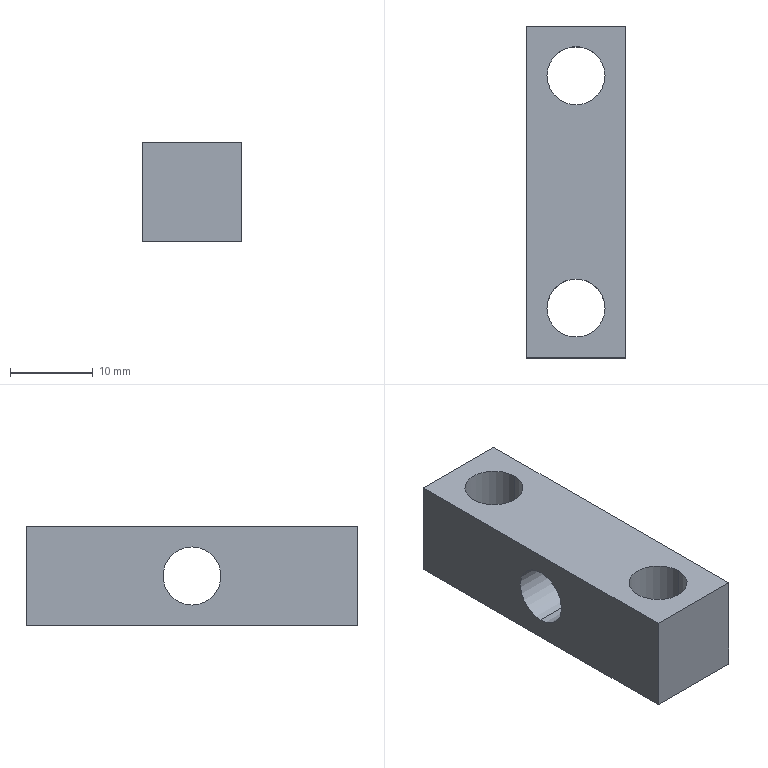Part | SolidWorks | features Extrusion 1, ICE 1 | 1 solid | 12 faces | box 12 x 40 x 12 mm | volume 4375 mm3 | cylinder 6 | plane 6 | commonest cylinder face diameters 7 x6
STEP:
#1=CARTESIAN_POINT('',(-6.,0.,-3.5));
#2=VERTEX_POINT('',#1);
#3=CARTESIAN_POINT('',(-6.,0.,3.5));
#4=VERTEX_POINT('',#3);
#5=CARTESIAN_POINT('',(-6.,0.,0.));
#6=DIRECTION('',(-1.,0.,0.));
#7=DIRECTION('',(0.,0.,-1.));
#8=AXIS2_PLACEMENT_3D('',#5,#6,#7);
#9=CIRCLE('',#8,3.5);
#10=EDGE_CURVE('',#2,#4,#9,.T.);
#11=ORIENTED_EDGE('',*,*,#10,.T.);
#12=CARTESIAN_POINT('',(6.,0.,3.5));
#13=VERTEX_POINT('',#12);
#14=CARTESIAN_POINT('',(-6.001,0.,3.5));
#15=DIRECTION('',(1.,0.,0.));
#16=VECTOR('',#15,1000.);
#17=LINE('',#14,#16);
#18=EDGE_CURVE('',#4,#13,#17,.T.);
#19=ORIENTED_EDGE('',*,*,#18,.T.);
#20=CARTESIAN_POINT('',(6.,0.,-3.5));
#21=VERTEX_POINT('',#20);
#22=CARTESIAN_POINT('',(6.,0.,0.));
#23=DIRECTION('',(1.,0.,0.));
#24=DIRECTION('',(0.,0.,-1.));
#25=AXIS2_PLACEMENT_3D('',#22,#23,#24);
#26=CIRCLE('',#25,3.5);
#27=EDGE_CURVE('',#13,#21,#26,.T.);
#28=ORIENTED_EDGE('',*,*,#27,.T.);
#29=CARTESIAN_POINT('',(-6.001,0.,-3.5));
#30=DIRECTION('',(1.,0.,0.));
#31=VECTOR('',#30,1000.);
#32=LINE('',#29,#31);
#33=EDGE_CURVE('',#2,#21,#32,.T.);
#34=ORIENTED_EDGE('',*,*,#33,.F.);
#35=EDGE_LOOP('',(#11,#19,#28,#34));
#36=FACE_OUTER_BOUND('',#35,.T.);
#37=CARTESIAN_POINT('',(-6.001,0.,0.));
#38=DIRECTION('',(1.,0.,0.));
#39=DIRECTION('',(0.,0.,-1.));
#40=AXIS2_PLACEMENT_3D('',#37,#38,#39);
#41=CYLINDRICAL_SURFACE('',#40,3.5);
#42=ADVANCED_FACE('',(#36),#41,.F.);
#43=CARTESIAN_POINT('',(-3.5,-14.,6.));
#44=VERTEX_POINT('',#43);
#45=CARTESIAN_POINT('',(3.5,-14.,6.));
#46=VERTEX_POINT('',#45);
#47=CARTESIAN_POINT('',(0.,-14.,6.));
#48=DIRECTION('',(0.,0.,1.));
#49=DIRECTION('',(1.,0.,0.));
#50=AXIS2_PLACEMENT_3D('',#47,#48,#49);
#51=CIRCLE('',#50,3.5);
#52=EDGE_CURVE('',#44,#46,#51,.T.);
#53=ORIENTED_EDGE('',*,*,#52,.T.);
#54=CARTESIAN_POINT('',(3.5,-14.,-6.));
#55=VERTEX_POINT('',#54);
#56=CARTESIAN_POINT('',(3.5,-14.,6.));
#57=DIRECTION('',(0.,0.,-1.));
#58=VECTOR('',#57,1000.);
#59=LINE('',#56,#58);
#60=EDGE_CURVE('',#46,#55,#59,.T.);
#61=ORIENTED_EDGE('',*,*,#60,.T.);
#62=CARTESIAN_POINT('',(-3.5,-14.,-6.));
#63=VERTEX_POINT('',#62);
#64=CARTESIAN_POINT('',(0.,-14.,-6.));
#65=DIRECTION('',(0.,0.,1.));
#66=DIRECTION('',(1.,0.,0.));
#67=AXIS2_PLACEMENT_3D('',#64,#65,#66);
#68=CIRCLE('',#67,3.5);
#69=EDGE_CURVE('',#63,#55,#68,.T.);
#70=ORIENTED_EDGE('',*,*,#69,.F.);
#71=CARTESIAN_POINT('',(-3.5,-14.,6.));
#72=DIRECTION('',(0.,0.,-1.));
#73=VECTOR('',#72,1000.);
#74=LINE('',#71,#73);
#75=EDGE_CURVE('',#44,#63,#74,.T.);
#76=ORIENTED_EDGE('',*,*,#75,.F.);
#77=EDGE_LOOP('',(#53,#61,#70,#76));
#78=FACE_OUTER_BOUND('',#77,.T.);
#79=CARTESIAN_POINT('',(0.,-14.,6.));
#80=DIRECTION('',(0.,0.,-1.));
#81=DIRECTION('',(-1.,0.,0.));
#82=AXIS2_PLACEMENT_3D('',#79,#80,#81);
#83=CYLINDRICAL_SURFACE('',#82,3.5);
#84=ADVANCED_FACE('',(#78),#83,.F.);
#85=CARTESIAN_POINT('',(-3.5,14.,6.));
#86=VERTEX_POINT('',#85);
#87=CARTESIAN_POINT('',(3.5,14.,6.));
#88=VERTEX_POINT('',#87);
#89=CARTESIAN_POINT('',(0.,14.,6.));
#90=DIRECTION('',(0.,0.,1.));
#91=DIRECTION('',(1.,0.,0.));
#92=AXIS2_PLACEMENT_3D('',#89,#90,#91);
#93=CIRCLE('',#92,3.5);
#94=EDGE_CURVE('',#86,#88,#93,.T.);
#95=ORIENTED_EDGE('',*,*,#94,.T.);
#96=CARTESIAN_POINT('',(3.5,14.,-6.));
#97=VERTEX_POINT('',#96);
#98=CARTESIAN_POINT('',(3.5,14.,6.));
#99=DIRECTION('',(0.,0.,-1.));
#100=VECTOR('',#99,1000.);
#101=LINE('',#98,#100);
#102=EDGE_CURVE('',#88,#97,#101,.T.);
#103=ORIENTED_EDGE('',*,*,#102,.T.);
#104=CARTESIAN_POINT('',(-3.5,14.,-6.));
#105=VERTEX_POINT('',#104);
#106=CARTESIAN_POINT('',(0.,14.,-6.));
#107=DIRECTION('',(0.,0.,1.));
#108=DIRECTION('',(1.,0.,0.));
#109=AXIS2_PLACEMENT_3D('',#106,#107,#108);
#110=CIRCLE('',#109,3.5);
#111=EDGE_CURVE('',#105,#97,#110,.T.);
#112=ORIENTED_EDGE('',*,*,#111,.F.);
#113=CARTESIAN_POINT('',(-3.5,14.,6.));
#114=DIRECTION('',(0.,0.,-1.));
#115=VECTOR('',#114,1000.);
#116=LINE('',#113,#115);
#117=EDGE_CURVE('',#86,#105,#116,.T.);
#118=ORIENTED_EDGE('',*,*,#117,.F.);
#119=EDGE_LOOP('',(#95,#103,#112,#118));
#120=FACE_OUTER_BOUND('',#119,.T.);
#121=CARTESIAN_POINT('',(0.,14.,6.));
#122=DIRECTION('',(0.,0.,-1.));
#123=DIRECTION('',(-1.,0.,0.));
#124=AXIS2_PLACEMENT_3D('',#121,#122,#123);
#125=CYLINDRICAL_SURFACE('',#124,3.5);
#126=ADVANCED_FACE('',(#120),#125,.F.);
#127=CARTESIAN_POINT('',(6.,-20.,6.));
#128=VERTEX_POINT('',#127);
#129=CARTESIAN_POINT('',(6.,20.,6.));
#130=VERTEX_POINT('',#129);
#131=CARTESIAN_POINT('',(6.,-20.,6.));
#132=DIRECTION('',(0.,1.,0.));
#133=VECTOR('',#132,1000.);
#134=LINE('',#131,#133);
#135=EDGE_CURVE('',#128,#130,#134,.T.);
#136=ORIENTED_EDGE('',*,*,#135,.T.);
#137=CARTESIAN_POINT('',(-6.,20.,6.));
#138=VERTEX_POINT('',#137);
#139=CARTESIAN_POINT('',(-6.,20.,6.));
#140=DIRECTION('',(-1.,0.,0.));
#141=VECTOR('',#140,1000.);
#142=LINE('',#139,#141);
#143=EDGE_CURVE('',#130,#138,#142,.T.);
#144=ORIENTED_EDGE('',*,*,#143,.T.);
#145=CARTESIAN_POINT('',(-6.,-20.,6.));
#146=VERTEX_POINT('',#145);
#147=CARTESIAN_POINT('',(-6.,-20.,6.));
#148=DIRECTION('',(0.,-1.,0.));
#149=VECTOR('',#148,1000.);
#150=LINE('',#147,#149);
#151=EDGE_CURVE('',#138,#146,#150,.T.);
#152=ORIENTED_EDGE('',*,*,#151,.T.);
#153=CARTESIAN_POINT('',(-6.,-20.,6.));
#154=DIRECTION('',(1.,0.,0.));
#155=VECTOR('',#154,1000.);
#156=LINE('',#153,#155);
#157=EDGE_CURVE('',#146,#128,#156,.T.);
#158=ORIENTED_EDGE('',*,*,#157,.T.);
#159=EDGE_LOOP('',(#136,#144,#152,#158));
#160=FACE_OUTER_BOUND('',#159,.T.);
#161=ORIENTED_EDGE('',*,*,#94,.F.);
#162=CARTESIAN_POINT('',(0.,14.,6.));
#163=DIRECTION('',(0.,0.,1.));
#164=DIRECTION('',(1.,0.,0.));
#165=AXIS2_PLACEMENT_3D('',#162,#163,#164);
#166=CIRCLE('',#165,3.5);
#167=EDGE_CURVE('',#88,#86,#166,.T.);
#168=ORIENTED_EDGE('',*,*,#167,.F.);
#169=EDGE_LOOP('',(#161,#168));
#170=FACE_BOUND('',#169,.T.);
#171=ORIENTED_EDGE('',*,*,#52,.F.);
#172=CARTESIAN_POINT('',(0.,-14.,6.));
#173=DIRECTION('',(0.,0.,1.));
#174=DIRECTION('',(1.,0.,0.));
#175=AXIS2_PLACEMENT_3D('',#172,#173,#174);
#176=CIRCLE('',#175,3.5);
#177=EDGE_CURVE('',#46,#44,#176,.T.);
#178=ORIENTED_EDGE('',*,*,#177,.F.);
#179=EDGE_LOOP('',(#171,#178));
#180=FACE_BOUND('',#179,.T.);
#181=CARTESIAN_POINT('',(0.,0.,6.));
#182=DIRECTION('',(0.,0.,-1.));
#183=DIRECTION('',(-1.,0.,0.));
#184=AXIS2_PLACEMENT_3D('',#181,#182,#183);
#185=PLANE('',#184);
#186=ADVANCED_FACE('',(#160,#170,#180),#185,.F.);
#187=ORIENTED_EDGE('',*,*,#111,.T.);
#188=CARTESIAN_POINT('',(0.,14.,-6.));
#189=DIRECTION('',(0.,0.,1.));
#190=DIRECTION('',(1.,0.,0.));
#191=AXIS2_PLACEMENT_3D('',#188,#189,#190);
#192=CIRCLE('',#191,3.5);
#193=EDGE_CURVE('',#97,#105,#192,.T.);
#194=ORIENTED_EDGE('',*,*,#193,.T.);
#195=EDGE_LOOP('',(#187,#194));
#196=FACE_BOUND('',#195,.T.);
#197=CARTESIAN_POINT('',(6.,-20.,-6.));
#198=VERTEX_POINT('',#197);
#199=CARTESIAN_POINT('',(6.,20.,-6.));
#200=VERTEX_POINT('',#199);
#201=CARTESIAN_POINT('',(6.,-20.,-6.));
#202=DIRECTION('',(0.,1.,0.));
#203=VECTOR('',#202,1000.);
#204=LINE('',#201,#203);
#205=EDGE_CURVE('',#198,#200,#204,.T.);
#206=ORIENTED_EDGE('',*,*,#205,.F.);
#207=CARTESIAN_POINT('',(-6.,-20.,-6.));
#208=VERTEX_POINT('',#207);
#209=CARTESIAN_POINT('',(-6.,-20.,-6.));
#210=DIRECTION('',(1.,0.,0.));
#211=VECTOR('',#210,1000.);
#212=LINE('',#209,#211);
#213=EDGE_CURVE('',#208,#198,#212,.T.);
#214=ORIENTED_EDGE('',*,*,#213,.F.);
#215=CARTESIAN_POINT('',(-6.,20.,-6.));
#216=VERTEX_POINT('',#215);
#217=CARTESIAN_POINT('',(-6.,-20.,-6.));
#218=DIRECTION('',(0.,-1.,0.));
#219=VECTOR('',#218,1000.);
#220=LINE('',#217,#219);
#221=EDGE_CURVE('',#216,#208,#220,.T.);
#222=ORIENTED_EDGE('',*,*,#221,.F.);
#223=CARTESIAN_POINT('',(-6.,20.,-6.));
#224=DIRECTION('',(-1.,0.,0.));
#225=VECTOR('',#224,1000.);
#226=LINE('',#223,#225);
#227=EDGE_CURVE('',#200,#216,#226,.T.);
#228=ORIENTED_EDGE('',*,*,#227,.F.);
#229=EDGE_LOOP('',(#206,#214,#222,#228));
#230=FACE_OUTER_BOUND('',#229,.T.);
#231=ORIENTED_EDGE('',*,*,#69,.T.);
#232=CARTESIAN_POINT('',(0.,-14.,-6.));
#233=DIRECTION('',(0.,0.,1.));
#234=DIRECTION('',(1.,0.,0.));
#235=AXIS2_PLACEMENT_3D('',#232,#233,#234);
#236=CIRCLE('',#235,3.5);
#237=EDGE_CURVE('',#55,#63,#236,.T.);
#238=ORIENTED_EDGE('',*,*,#237,.T.);
#239=EDGE_LOOP('',(#231,#238));
#240=FACE_BOUND('',#239,.T.);
#241=CARTESIAN_POINT('',(0.,0.,-6.));
#242=DIRECTION('',(0.,0.,-1.));
#243=DIRECTION('',(-1.,0.,0.));
#244=AXIS2_PLACEMENT_3D('',#241,#242,#243);
#245=PLANE('',#244);
#246=ADVANCED_FACE('',(#196,#230,#240),#245,.T.);
#247=CARTESIAN_POINT('',(6.,0.,0.));
#248=DIRECTION('',(1.,0.,0.));
#249=DIRECTION('',(0.,0.,-1.));
#250=AXIS2_PLACEMENT_3D('',#247,#248,#249);
#251=CIRCLE('',#250,3.5);
#252=EDGE_CURVE('',#21,#13,#251,.T.);
#253=ORIENTED_EDGE('',*,*,#252,.F.);
#254=ORIENTED_EDGE('',*,*,#27,.F.);
#255=EDGE_LOOP('',(#253,#254));
#256=FACE_BOUND('',#255,.T.);
#257=ORIENTED_EDGE('',*,*,#205,.T.);
#258=CARTESIAN_POINT('',(6.,20.,6.));
#259=DIRECTION('',(0.,0.,-1.));
#260=VECTOR('',#259,1000.);
#261=LINE('',#258,#260);
#262=EDGE_CURVE('',#130,#200,#261,.T.);
#263=ORIENTED_EDGE('',*,*,#262,.F.);
#264=ORIENTED_EDGE('',*,*,#135,.F.);
#265=CARTESIAN_POINT('',(6.,-20.,6.));
#266=DIRECTION('',(0.,0.,-1.));
#267=VECTOR('',#266,1000.);
#268=LINE('',#265,#267);
#269=EDGE_CURVE('',#128,#198,#268,.T.);
#270=ORIENTED_EDGE('',*,*,#269,.T.);
#271=EDGE_LOOP('',(#257,#263,#264,#270));
#272=FACE_OUTER_BOUND('',#271,.T.);
#273=CARTESIAN_POINT('',(6.,-20.,6.));
#274=DIRECTION('',(-1.,0.,0.));
#275=DIRECTION('',(0.,0.,1.));
#276=AXIS2_PLACEMENT_3D('',#273,#274,#275);
#277=PLANE('',#276);
#278=ADVANCED_FACE('',(#256,#272),#277,.F.);
#279=ORIENTED_EDGE('',*,*,#227,.T.);
#280=CARTESIAN_POINT('',(-6.,20.,6.));
#281=DIRECTION('',(0.,0.,-1.));
#282=VECTOR('',#281,1000.);
#283=LINE('',#280,#282);
#284=EDGE_CURVE('',#138,#216,#283,.T.);
#285=ORIENTED_EDGE('',*,*,#284,.F.);
#286=ORIENTED_EDGE('',*,*,#143,.F.);
#287=ORIENTED_EDGE('',*,*,#262,.T.);
#288=EDGE_LOOP('',(#279,#285,#286,#287));
#289=FACE_OUTER_BOUND('',#288,.T.);
#290=CARTESIAN_POINT('',(-6.,20.,6.));
#291=DIRECTION('',(0.,-1.,0.));
#292=DIRECTION('',(0.,0.,-1.));
#293=AXIS2_PLACEMENT_3D('',#290,#291,#292);
#294=PLANE('',#293);
#295=ADVANCED_FACE('',(#289),#294,.F.);
#296=ORIENTED_EDGE('',*,*,#10,.F.);
#297=CARTESIAN_POINT('',(-6.,0.,0.));
#298=DIRECTION('',(-1.,0.,0.));
#299=DIRECTION('',(0.,0.,-1.));
#300=AXIS2_PLACEMENT_3D('',#297,#298,#299);
#301=CIRCLE('',#300,3.5);
#302=EDGE_CURVE('',#4,#2,#301,.T.);
#303=ORIENTED_EDGE('',*,*,#302,.F.);
#304=EDGE_LOOP('',(#296,#303));
#305=FACE_BOUND('',#304,.T.);
#306=ORIENTED_EDGE('',*,*,#221,.T.);
#307=CARTESIAN_POINT('',(-6.,-20.,6.));
#308=DIRECTION('',(0.,0.,-1.));
#309=VECTOR('',#308,1000.);
#310=LINE('',#307,#309);
#311=EDGE_CURVE('',#146,#208,#310,.T.);
#312=ORIENTED_EDGE('',*,*,#311,.F.);
#313=ORIENTED_EDGE('',*,*,#151,.F.);
#314=ORIENTED_EDGE('',*,*,#284,.T.);
#315=EDGE_LOOP('',(#306,#312,#313,#314));
#316=FACE_OUTER_BOUND('',#315,.T.);
#317=CARTESIAN_POINT('',(-6.,-20.,6.));
#318=DIRECTION('',(1.,0.,0.));
#319=DIRECTION('',(0.,0.,-1.));
#320=AXIS2_PLACEMENT_3D('',#317,#318,#319);
#321=PLANE('',#320);
#322=ADVANCED_FACE('',(#305,#316),#321,.F.);
#323=ORIENTED_EDGE('',*,*,#213,.T.);
#324=ORIENTED_EDGE('',*,*,#269,.F.);
#325=ORIENTED_EDGE('',*,*,#157,.F.);
#326=ORIENTED_EDGE('',*,*,#311,.T.);
#327=EDGE_LOOP('',(#323,#324,#325,#326));
#328=FACE_OUTER_BOUND('',#327,.T.);
#329=CARTESIAN_POINT('',(-6.,-20.,6.));
#330=DIRECTION('',(0.,1.,0.));
#331=DIRECTION('',(0.,0.,1.));
#332=AXIS2_PLACEMENT_3D('',#329,#330,#331);
#333=PLANE('',#332);
#334=ADVANCED_FACE('',(#328),#333,.F.);
#335=ORIENTED_EDGE('',*,*,#102,.F.);
#336=ORIENTED_EDGE('',*,*,#167,.T.);
#337=ORIENTED_EDGE('',*,*,#117,.T.);
#338=ORIENTED_EDGE('',*,*,#193,.F.);
#339=EDGE_LOOP('',(#335,#336,#337,#338));
#340=FACE_OUTER_BOUND('',#339,.T.);
#341=CARTESIAN_POINT('',(0.,14.,6.));
#342=DIRECTION('',(0.,0.,-1.));
#343=DIRECTION('',(-1.,0.,0.));
#344=AXIS2_PLACEMENT_3D('',#341,#342,#343);
#345=CYLINDRICAL_SURFACE('',#344,3.5);
#346=ADVANCED_FACE('',(#340),#345,.F.);
#347=ORIENTED_EDGE('',*,*,#60,.F.);
#348=ORIENTED_EDGE('',*,*,#177,.T.);
#349=ORIENTED_EDGE('',*,*,#75,.T.);
#350=ORIENTED_EDGE('',*,*,#237,.F.);
#351=EDGE_LOOP('',(#347,#348,#349,#350));
#352=FACE_OUTER_BOUND('',#351,.T.);
#353=CARTESIAN_POINT('',(0.,-14.,6.));
#354=DIRECTION('',(0.,0.,-1.));
#355=DIRECTION('',(-1.,0.,0.));
#356=AXIS2_PLACEMENT_3D('',#353,#354,#355);
#357=CYLINDRICAL_SURFACE('',#356,3.5);
#358=ADVANCED_FACE('',(#352),#357,.F.);
#359=ORIENTED_EDGE('',*,*,#18,.F.);
#360=ORIENTED_EDGE('',*,*,#302,.T.);
#361=ORIENTED_EDGE('',*,*,#33,.T.);
#362=ORIENTED_EDGE('',*,*,#252,.T.);
#363=EDGE_LOOP('',(#359,#360,#361,#362));
#364=FACE_OUTER_BOUND('',#363,.T.);
#365=CARTESIAN_POINT('',(-6.001,0.,0.));
#366=DIRECTION('',(1.,0.,0.));
#367=DIRECTION('',(0.,0.,-1.));
#368=AXIS2_PLACEMENT_3D('',#365,#366,#367);
#369=CYLINDRICAL_SURFACE('',#368,3.5);
#370=ADVANCED_FACE('',(#364),#369,.F.);
#371=CLOSED_SHELL('',(#42,#84,#126,#186,#246,#278,#295,#322,#334,#346,#358,#370));
#372=MANIFOLD_SOLID_BREP('',#371);
#373=CARTESIAN_POINT('',(0.,0.,0.));
#374=DIRECTION('',(0.,0.,1.));
#375=DIRECTION('',(1.,0.,0.));
#376=AXIS2_PLACEMENT_3D('',#373,#374,#375);
#377=(LENGTH_UNIT()NAMED_UNIT(*)SI_UNIT(.MILLI.,.METRE.));
#378=UNCERTAINTY_MEASURE_WITH_UNIT(LENGTH_MEASURE(0.00001),#377,'','');
#379=(NAMED_UNIT(*)PLANE_ANGLE_UNIT()SI_UNIT($,.RADIAN.));
#380=(NAMED_UNIT(*)SI_UNIT($,.STERADIAN.)SOLID_ANGLE_UNIT());
#381=(GEOMETRIC_REPRESENTATION_CONTEXT(3)GLOBAL_UNCERTAINTY_ASSIGNED_CONTEXT((#378))GLOBAL_UNIT_ASSIGNED_CONTEXT((#377,#379,#380))REPRESENTATION_CONTEXT('',''));
#382=ADVANCED_BREP_SHAPE_REPRESENTATION('',(#372,#376),#381);